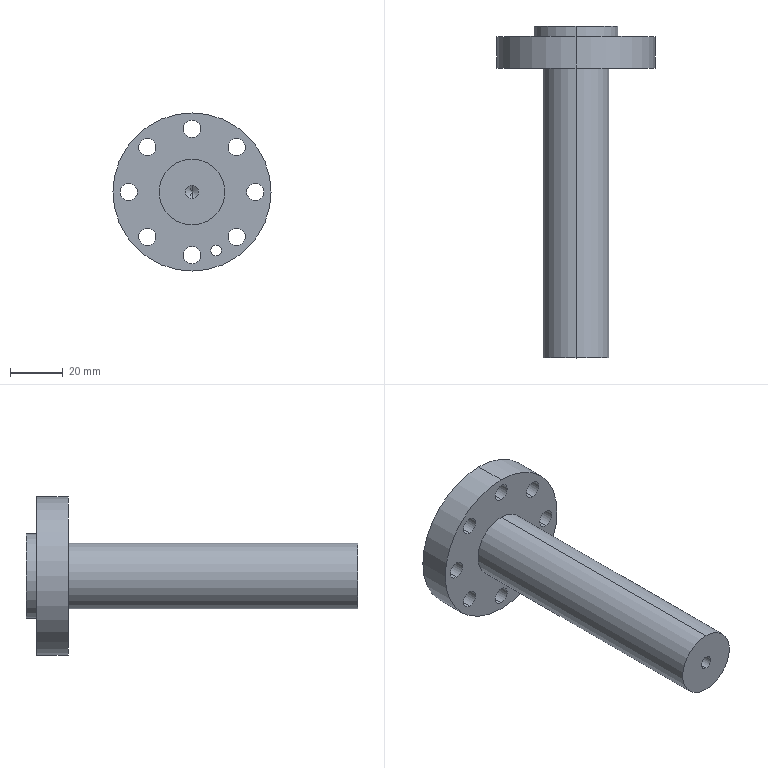Part | SolidWorks | features HoleWzd 3, Cut 1, Extrusion 1, ICE 1 | 1 solid | 32 faces | box 60 x 126 x 60 mm | volume 87403 mm3 | cylinder 26 | plane 4 | cone 2 | commonest cylinder face diameters 6.6 x16 4 x2 5 x2 25 x2 32 x2 60 x2
STEP:
#1=CARTESIAN_POINT('',(0.,15.,2.5));
#2=VERTEX_POINT('',#1);
#3=CARTESIAN_POINT('',(0.,15.,-2.5));
#4=VERTEX_POINT('',#3);
#5=CARTESIAN_POINT('',(0.,15.,0.));
#6=DIRECTION('',(0.,-1.,0.));
#7=DIRECTION('',(0.,0.,-1.));
#8=AXIS2_PLACEMENT_3D('',#5,#6,#7);
#9=CIRCLE('',#8,2.5);
#10=EDGE_CURVE('',#2,#4,#9,.T.);
#11=ORIENTED_EDGE('',*,*,#10,.F.);
#12=CARTESIAN_POINT('',(0.,0.,2.5));
#13=VERTEX_POINT('',#12);
#14=CARTESIAN_POINT('',(0.,0.,2.5));
#15=DIRECTION('',(0.,-1.,0.));
#16=VECTOR('',#15,1000.);
#17=LINE('',#14,#16);
#18=EDGE_CURVE('',#2,#13,#17,.T.);
#19=ORIENTED_EDGE('',*,*,#18,.T.);
#20=CARTESIAN_POINT('',(0.,0.,-2.5));
#21=VERTEX_POINT('',#20);
#22=CARTESIAN_POINT('',(0.,0.,0.));
#23=DIRECTION('',(0.,-1.,0.));
#24=DIRECTION('',(0.,0.,-1.));
#25=AXIS2_PLACEMENT_3D('',#22,#23,#24);
#26=CIRCLE('',#25,2.5);
#27=EDGE_CURVE('',#13,#21,#26,.T.);
#28=ORIENTED_EDGE('',*,*,#27,.T.);
#29=CARTESIAN_POINT('',(0.,0.,-2.5));
#30=DIRECTION('',(0.,-1.,0.));
#31=VECTOR('',#30,1000.);
#32=LINE('',#29,#31);
#33=EDGE_CURVE('',#4,#21,#32,.T.);
#34=ORIENTED_EDGE('',*,*,#33,.F.);
#35=EDGE_LOOP('',(#11,#19,#28,#34));
#36=FACE_OUTER_BOUND('',#35,.T.);
#37=CARTESIAN_POINT('',(0.,0.,0.));
#38=DIRECTION('',(0.,-1.,0.));
#39=DIRECTION('',(0.,0.,-1.));
#40=AXIS2_PLACEMENT_3D('',#37,#38,#39);
#41=CYLINDRICAL_SURFACE('',#40,2.5);
#42=ADVANCED_FACE('',(#36),#41,.F.);
#43=CARTESIAN_POINT('',(0.,16.502,0.));
#44=VERTEX_POINT('',#43);
#45=CARTESIAN_POINT('',(0.,15.,-2.5));
#46=DIRECTION('',(0.,-0.515,-0.8572));
#47=VECTOR('',#46,1000.);
#48=LINE('',#45,#47);
#49=EDGE_CURVE('',#44,#4,#48,.T.);
#50=ORIENTED_EDGE('',*,*,#49,.F.);
#51=CARTESIAN_POINT('',(0.,15.,2.5));
#52=DIRECTION('',(0.,-0.515,0.8572));
#53=VECTOR('',#52,1000.);
#54=LINE('',#51,#53);
#55=EDGE_CURVE('',#44,#2,#54,.T.);
#56=ORIENTED_EDGE('',*,*,#55,.T.);
#57=ORIENTED_EDGE('',*,*,#10,.T.);
#58=EDGE_LOOP('',(#50,#56,#57));
#59=FACE_OUTER_BOUND('',#58,.T.);
#60=CARTESIAN_POINT('',(0.,15.,0.));
#61=DIRECTION('',(0.,-1.,0.));
#62=DIRECTION('',(0.,0.,-1.));
#63=AXIS2_PLACEMENT_3D('',#60,#61,#62);
#64=CONICAL_SURFACE('',#63,2.5,1.03);
#65=ADVANCED_FACE('',(#59),#64,.F.);
#66=CARTESIAN_POINT('',(9.184,122.,-24.173));
#67=VERTEX_POINT('',#66);
#68=CARTESIAN_POINT('',(9.184,122.,-20.173));
#69=VERTEX_POINT('',#68);
#70=CARTESIAN_POINT('',(9.184,122.,-22.173));
#71=DIRECTION('',(0.,1.,0.));
#72=DIRECTION('',(0.,0.,1.));
#73=AXIS2_PLACEMENT_3D('',#70,#71,#72);
#74=CIRCLE('',#73,2.);
#75=EDGE_CURVE('',#67,#69,#74,.T.);
#76=ORIENTED_EDGE('',*,*,#75,.T.);
#77=CARTESIAN_POINT('',(9.184,110.,-20.173));
#78=VERTEX_POINT('',#77);
#79=CARTESIAN_POINT('',(9.184,110.,-20.173));
#80=DIRECTION('',(0.,-1.,0.));
#81=VECTOR('',#80,1000.);
#82=LINE('',#79,#81);
#83=EDGE_CURVE('',#69,#78,#82,.T.);
#84=ORIENTED_EDGE('',*,*,#83,.T.);
#85=CARTESIAN_POINT('',(9.184,110.,-24.173));
#86=VERTEX_POINT('',#85);
#87=CARTESIAN_POINT('',(9.184,110.,-22.173));
#88=DIRECTION('',(0.,-1.,0.));
#89=DIRECTION('',(0.,0.,-1.));
#90=AXIS2_PLACEMENT_3D('',#87,#88,#89);
#91=CIRCLE('',#90,2.);
#92=EDGE_CURVE('',#78,#86,#91,.T.);
#93=ORIENTED_EDGE('',*,*,#92,.T.);
#94=CARTESIAN_POINT('',(9.184,110.,-24.173));
#95=DIRECTION('',(0.,-1.,0.));
#96=VECTOR('',#95,1000.);
#97=LINE('',#94,#96);
#98=EDGE_CURVE('',#67,#86,#97,.T.);
#99=ORIENTED_EDGE('',*,*,#98,.F.);
#100=EDGE_LOOP('',(#76,#84,#93,#99));
#101=FACE_OUTER_BOUND('',#100,.T.);
#102=CARTESIAN_POINT('',(9.184,110.,-22.173));
#103=DIRECTION('',(0.,-1.,0.));
#104=DIRECTION('',(0.,0.,-1.));
#105=AXIS2_PLACEMENT_3D('',#102,#103,#104);
#106=CYLINDRICAL_SURFACE('',#105,2.);
#107=ADVANCED_FACE('',(#101),#106,.F.);
#108=CARTESIAN_POINT('',(0.,126.,16.));
#109=VERTEX_POINT('',#108);
#110=CARTESIAN_POINT('',(0.,126.,-16.));
#111=VERTEX_POINT('',#110);
#112=CARTESIAN_POINT('',(0.,126.,0.));
#113=DIRECTION('',(0.,1.,0.));
#114=DIRECTION('',(0.,0.,1.));
#115=AXIS2_PLACEMENT_3D('',#112,#113,#114);
#116=CIRCLE('',#115,16.);
#117=EDGE_CURVE('',#109,#111,#116,.T.);
#118=ORIENTED_EDGE('',*,*,#117,.F.);
#119=CARTESIAN_POINT('',(0.,122.,16.));
#120=VERTEX_POINT('',#119);
#121=CARTESIAN_POINT('',(0.,126.,16.));
#122=DIRECTION('',(0.,-1.,0.));
#123=VECTOR('',#122,1000.);
#124=LINE('',#121,#123);
#125=EDGE_CURVE('',#109,#120,#124,.T.);
#126=ORIENTED_EDGE('',*,*,#125,.T.);
#127=CARTESIAN_POINT('',(0.,122.,-16.));
#128=VERTEX_POINT('',#127);
#129=CARTESIAN_POINT('',(0.,122.,0.));
#130=DIRECTION('',(0.,1.,0.));
#131=DIRECTION('',(0.,0.,1.));
#132=AXIS2_PLACEMENT_3D('',#129,#130,#131);
#133=CIRCLE('',#132,16.);
#134=EDGE_CURVE('',#120,#128,#133,.T.);
#135=ORIENTED_EDGE('',*,*,#134,.T.);
#136=CARTESIAN_POINT('',(0.,126.,-16.));
#137=DIRECTION('',(0.,-1.,0.));
#138=VECTOR('',#137,1000.);
#139=LINE('',#136,#138);
#140=EDGE_CURVE('',#111,#128,#139,.T.);
#141=ORIENTED_EDGE('',*,*,#140,.F.);
#142=EDGE_LOOP('',(#118,#126,#135,#141));
#143=FACE_OUTER_BOUND('',#142,.T.);
#144=CARTESIAN_POINT('',(0.,126.,0.));
#145=DIRECTION('',(0.,-1.,0.));
#146=DIRECTION('',(0.,0.,-1.));
#147=AXIS2_PLACEMENT_3D('',#144,#145,#146);
#148=CYLINDRICAL_SURFACE('',#147,16.);
#149=ADVANCED_FACE('',(#143),#148,.T.);
#150=CARTESIAN_POINT('',(24.,122.,3.3));
#151=VERTEX_POINT('',#150);
#152=CARTESIAN_POINT('',(24.,122.,-3.3));
#153=VERTEX_POINT('',#152);
#154=CARTESIAN_POINT('',(24.,122.,0.));
#155=DIRECTION('',(0.,-1.,0.));
#156=DIRECTION('',(0.,0.,-1.));
#157=AXIS2_PLACEMENT_3D('',#154,#155,#156);
#158=CIRCLE('',#157,3.3);
#159=EDGE_CURVE('',#151,#153,#158,.T.);
#160=ORIENTED_EDGE('',*,*,#159,.F.);
#161=CARTESIAN_POINT('',(24.,110.,3.3));
#162=VERTEX_POINT('',#161);
#163=CARTESIAN_POINT('',(24.,110.,3.3));
#164=DIRECTION('',(0.,-1.,0.));
#165=VECTOR('',#164,1000.);
#166=LINE('',#163,#165);
#167=EDGE_CURVE('',#151,#162,#166,.T.);
#168=ORIENTED_EDGE('',*,*,#167,.T.);
#169=CARTESIAN_POINT('',(24.,110.,-3.3));
#170=VERTEX_POINT('',#169);
#171=CARTESIAN_POINT('',(24.,110.,0.));
#172=DIRECTION('',(0.,-1.,0.));
#173=DIRECTION('',(0.,0.,-1.));
#174=AXIS2_PLACEMENT_3D('',#171,#172,#173);
#175=CIRCLE('',#174,3.3);
#176=EDGE_CURVE('',#162,#170,#175,.T.);
#177=ORIENTED_EDGE('',*,*,#176,.T.);
#178=CARTESIAN_POINT('',(24.,110.,-3.3));
#179=DIRECTION('',(0.,-1.,0.));
#180=VECTOR('',#179,1000.);
#181=LINE('',#178,#180);
#182=EDGE_CURVE('',#153,#170,#181,.T.);
#183=ORIENTED_EDGE('',*,*,#182,.F.);
#184=EDGE_LOOP('',(#160,#168,#177,#183));
#185=FACE_OUTER_BOUND('',#184,.T.);
#186=CARTESIAN_POINT('',(24.,110.,0.));
#187=DIRECTION('',(0.,-1.,0.));
#188=DIRECTION('',(0.,0.,-1.));
#189=AXIS2_PLACEMENT_3D('',#186,#187,#188);
#190=CYLINDRICAL_SURFACE('',#189,3.3);
#191=ADVANCED_FACE('',(#185),#190,.F.);
#192=CARTESIAN_POINT('',(16.971,122.,-13.671));
#193=VERTEX_POINT('',#192);
#194=CARTESIAN_POINT('',(16.971,122.,-20.271));
#195=VERTEX_POINT('',#194);
#196=CARTESIAN_POINT('',(16.971,122.,-16.971));
#197=DIRECTION('',(0.,-1.,0.));
#198=DIRECTION('',(0.,0.,-1.));
#199=AXIS2_PLACEMENT_3D('',#196,#197,#198);
#200=CIRCLE('',#199,3.3);
#201=EDGE_CURVE('',#193,#195,#200,.T.);
#202=ORIENTED_EDGE('',*,*,#201,.F.);
#203=CARTESIAN_POINT('',(16.971,110.,-13.671));
#204=VERTEX_POINT('',#203);
#205=CARTESIAN_POINT('',(16.971,110.,-13.671));
#206=DIRECTION('',(0.,-1.,0.));
#207=VECTOR('',#206,1000.);
#208=LINE('',#205,#207);
#209=EDGE_CURVE('',#193,#204,#208,.T.);
#210=ORIENTED_EDGE('',*,*,#209,.T.);
#211=CARTESIAN_POINT('',(16.971,110.,-20.271));
#212=VERTEX_POINT('',#211);
#213=CARTESIAN_POINT('',(16.971,110.,-16.971));
#214=DIRECTION('',(0.,-1.,0.));
#215=DIRECTION('',(0.,0.,-1.));
#216=AXIS2_PLACEMENT_3D('',#213,#214,#215);
#217=CIRCLE('',#216,3.3);
#218=EDGE_CURVE('',#204,#212,#217,.T.);
#219=ORIENTED_EDGE('',*,*,#218,.T.);
#220=CARTESIAN_POINT('',(16.971,110.,-20.271));
#221=DIRECTION('',(0.,-1.,0.));
#222=VECTOR('',#221,1000.);
#223=LINE('',#220,#222);
#224=EDGE_CURVE('',#195,#212,#223,.T.);
#225=ORIENTED_EDGE('',*,*,#224,.F.);
#226=EDGE_LOOP('',(#202,#210,#219,#225));
#227=FACE_OUTER_BOUND('',#226,.T.);
#228=CARTESIAN_POINT('',(16.971,110.,-16.971));
#229=DIRECTION('',(0.,-1.,0.));
#230=DIRECTION('',(0.,0.,-1.));
#231=AXIS2_PLACEMENT_3D('',#228,#229,#230);
#232=CYLINDRICAL_SURFACE('',#231,3.3);
#233=ADVANCED_FACE('',(#227),#232,.F.);
#234=CARTESIAN_POINT('',(0.,122.,-20.7));
#235=VERTEX_POINT('',#234);
#236=CARTESIAN_POINT('',(0.,122.,-27.3));
#237=VERTEX_POINT('',#236);
#238=CARTESIAN_POINT('',(0.,122.,-24.));
#239=DIRECTION('',(0.,-1.,0.));
#240=DIRECTION('',(0.,0.,-1.));
#241=AXIS2_PLACEMENT_3D('',#238,#239,#240);
#242=CIRCLE('',#241,3.3);
#243=EDGE_CURVE('',#235,#237,#242,.T.);
#244=ORIENTED_EDGE('',*,*,#243,.F.);
#245=CARTESIAN_POINT('',(0.,110.,-20.7));
#246=VERTEX_POINT('',#245);
#247=CARTESIAN_POINT('',(0.,110.,-20.7));
#248=DIRECTION('',(0.,-1.,0.));
#249=VECTOR('',#248,1000.);
#250=LINE('',#247,#249);
#251=EDGE_CURVE('',#235,#246,#250,.T.);
#252=ORIENTED_EDGE('',*,*,#251,.T.);
#253=CARTESIAN_POINT('',(0.,110.,-27.3));
#254=VERTEX_POINT('',#253);
#255=CARTESIAN_POINT('',(0.,110.,-24.));
#256=DIRECTION('',(0.,-1.,0.));
#257=DIRECTION('',(0.,0.,-1.));
#258=AXIS2_PLACEMENT_3D('',#255,#256,#257);
#259=CIRCLE('',#258,3.3);
#260=EDGE_CURVE('',#246,#254,#259,.T.);
#261=ORIENTED_EDGE('',*,*,#260,.T.);
#262=CARTESIAN_POINT('',(0.,110.,-27.3));
#263=DIRECTION('',(0.,-1.,0.));
#264=VECTOR('',#263,1000.);
#265=LINE('',#262,#264);
#266=EDGE_CURVE('',#237,#254,#265,.T.);
#267=ORIENTED_EDGE('',*,*,#266,.F.);
#268=EDGE_LOOP('',(#244,#252,#261,#267));
#269=FACE_OUTER_BOUND('',#268,.T.);
#270=CARTESIAN_POINT('',(0.,110.,-24.));
#271=DIRECTION('',(0.,-1.,0.));
#272=DIRECTION('',(0.,0.,-1.));
#273=AXIS2_PLACEMENT_3D('',#270,#271,#272);
#274=CYLINDRICAL_SURFACE('',#273,3.3);
#275=ADVANCED_FACE('',(#269),#274,.F.);
#276=CARTESIAN_POINT('',(-16.971,122.,-13.671));
#277=VERTEX_POINT('',#276);
#278=CARTESIAN_POINT('',(-16.971,122.,-20.271));
#279=VERTEX_POINT('',#278);
#280=CARTESIAN_POINT('',(-16.971,122.,-16.971));
#281=DIRECTION('',(0.,-1.,0.));
#282=DIRECTION('',(0.,0.,-1.));
#283=AXIS2_PLACEMENT_3D('',#280,#281,#282);
#284=CIRCLE('',#283,3.3);
#285=EDGE_CURVE('',#277,#279,#284,.T.);
#286=ORIENTED_EDGE('',*,*,#285,.F.);
#287=CARTESIAN_POINT('',(-16.971,110.,-13.671));
#288=VERTEX_POINT('',#287);
#289=CARTESIAN_POINT('',(-16.971,110.,-13.671));
#290=DIRECTION('',(0.,-1.,0.));
#291=VECTOR('',#290,1000.);
#292=LINE('',#289,#291);
#293=EDGE_CURVE('',#277,#288,#292,.T.);
#294=ORIENTED_EDGE('',*,*,#293,.T.);
#295=CARTESIAN_POINT('',(-16.971,110.,-20.271));
#296=VERTEX_POINT('',#295);
#297=CARTESIAN_POINT('',(-16.971,110.,-16.971));
#298=DIRECTION('',(0.,-1.,0.));
#299=DIRECTION('',(0.,0.,-1.));
#300=AXIS2_PLACEMENT_3D('',#297,#298,#299);
#301=CIRCLE('',#300,3.3);
#302=EDGE_CURVE('',#288,#296,#301,.T.);
#303=ORIENTED_EDGE('',*,*,#302,.T.);
#304=CARTESIAN_POINT('',(-16.971,110.,-20.271));
#305=DIRECTION('',(0.,-1.,0.));
#306=VECTOR('',#305,1000.);
#307=LINE('',#304,#306);
#308=EDGE_CURVE('',#279,#296,#307,.T.);
#309=ORIENTED_EDGE('',*,*,#308,.F.);
#310=EDGE_LOOP('',(#286,#294,#303,#309));
#311=FACE_OUTER_BOUND('',#310,.T.);
#312=CARTESIAN_POINT('',(-16.971,110.,-16.971));
#313=DIRECTION('',(0.,-1.,0.));
#314=DIRECTION('',(0.,0.,-1.));
#315=AXIS2_PLACEMENT_3D('',#312,#313,#314);
#316=CYLINDRICAL_SURFACE('',#315,3.3);
#317=ADVANCED_FACE('',(#311),#316,.F.);
#318=CARTESIAN_POINT('',(-24.,122.,3.3));
#319=VERTEX_POINT('',#318);
#320=CARTESIAN_POINT('',(-24.,122.,-3.3));
#321=VERTEX_POINT('',#320);
#322=CARTESIAN_POINT('',(-24.,122.,0.));
#323=DIRECTION('',(0.,-1.,0.));
#324=DIRECTION('',(0.,0.,-1.));
#325=AXIS2_PLACEMENT_3D('',#322,#323,#324);
#326=CIRCLE('',#325,3.3);
#327=EDGE_CURVE('',#319,#321,#326,.T.);
#328=ORIENTED_EDGE('',*,*,#327,.F.);
#329=CARTESIAN_POINT('',(-24.,110.,3.3));
#330=VERTEX_POINT('',#329);
#331=CARTESIAN_POINT('',(-24.,110.,3.3));
#332=DIRECTION('',(0.,-1.,0.));
#333=VECTOR('',#332,1000.);
#334=LINE('',#331,#333);
#335=EDGE_CURVE('',#319,#330,#334,.T.);
#336=ORIENTED_EDGE('',*,*,#335,.T.);
#337=CARTESIAN_POINT('',(-24.,110.,-3.3));
#338=VERTEX_POINT('',#337);
#339=CARTESIAN_POINT('',(-24.,110.,0.));
#340=DIRECTION('',(0.,-1.,0.));
#341=DIRECTION('',(0.,0.,-1.));
#342=AXIS2_PLACEMENT_3D('',#339,#340,#341);
#343=CIRCLE('',#342,3.3);
#344=EDGE_CURVE('',#330,#338,#343,.T.);
#345=ORIENTED_EDGE('',*,*,#344,.T.);
#346=CARTESIAN_POINT('',(-24.,110.,-3.3));
#347=DIRECTION('',(0.,-1.,0.));
#348=VECTOR('',#347,1000.);
#349=LINE('',#346,#348);
#350=EDGE_CURVE('',#321,#338,#349,.T.);
#351=ORIENTED_EDGE('',*,*,#350,.F.);
#352=EDGE_LOOP('',(#328,#336,#345,#351));
#353=FACE_OUTER_BOUND('',#352,.T.);
#354=CARTESIAN_POINT('',(-24.,110.,0.));
#355=DIRECTION('',(0.,-1.,0.));
#356=DIRECTION('',(0.,0.,-1.));
#357=AXIS2_PLACEMENT_3D('',#354,#355,#356);
#358=CYLINDRICAL_SURFACE('',#357,3.3);
#359=ADVANCED_FACE('',(#353),#358,.F.);
#360=CARTESIAN_POINT('',(-16.971,122.,20.271));
#361=VERTEX_POINT('',#360);
#362=CARTESIAN_POINT('',(-16.971,122.,13.671));
#363=VERTEX_POINT('',#362);
#364=CARTESIAN_POINT('',(-16.971,122.,16.971));
#365=DIRECTION('',(0.,-1.,0.));
#366=DIRECTION('',(0.,0.,-1.));
#367=AXIS2_PLACEMENT_3D('',#364,#365,#366);
#368=CIRCLE('',#367,3.3);
#369=EDGE_CURVE('',#361,#363,#368,.T.);
#370=ORIENTED_EDGE('',*,*,#369,.F.);
#371=CARTESIAN_POINT('',(-16.971,110.,20.271));
#372=VERTEX_POINT('',#371);
#373=CARTESIAN_POINT('',(-16.971,110.,20.271));
#374=DIRECTION('',(0.,-1.,0.));
#375=VECTOR('',#374,1000.);
#376=LINE('',#373,#375);
#377=EDGE_CURVE('',#361,#372,#376,.T.);
#378=ORIENTED_EDGE('',*,*,#377,.T.);
#379=CARTESIAN_POINT('',(-16.971,110.,13.671));
#380=VERTEX_POINT('',#379);
#381=CARTESIAN_POINT('',(-16.971,110.,16.971));
#382=DIRECTION('',(0.,-1.,0.));
#383=DIRECTION('',(0.,0.,-1.));
#384=AXIS2_PLACEMENT_3D('',#381,#382,#383);
#385=CIRCLE('',#384,3.3);
#386=EDGE_CURVE('',#372,#380,#385,.T.);
#387=ORIENTED_EDGE('',*,*,#386,.T.);
#388=CARTESIAN_POINT('',(-16.971,110.,13.671));
#389=DIRECTION('',(0.,-1.,0.));
#390=VECTOR('',#389,1000.);
#391=LINE('',#388,#390);
#392=EDGE_CURVE('',#363,#380,#391,.T.);
#393=ORIENTED_EDGE('',*,*,#392,.F.);
#394=EDGE_LOOP('',(#370,#378,#387,#393));
#395=FACE_OUTER_BOUND('',#394,.T.);
#396=CARTESIAN_POINT('',(-16.971,110.,16.971));
#397=DIRECTION('',(0.,-1.,0.));
#398=DIRECTION('',(0.,0.,-1.));
#399=AXIS2_PLACEMENT_3D('',#396,#397,#398);
#400=CYLINDRICAL_SURFACE('',#399,3.3);
#401=ADVANCED_FACE('',(#395),#400,.F.);
#402=CARTESIAN_POINT('',(0.,122.,27.3));
#403=VERTEX_POINT('',#402);
#404=CARTESIAN_POINT('',(0.,122.,20.7));
#405=VERTEX_POINT('',#404);
#406=CARTESIAN_POINT('',(0.,122.,24.));
#407=DIRECTION('',(0.,-1.,0.));
#408=DIRECTION('',(0.,0.,-1.));
#409=AXIS2_PLACEMENT_3D('',#406,#407,#408);
#410=CIRCLE('',#409,3.3);
#411=EDGE_CURVE('',#403,#405,#410,.T.);
#412=ORIENTED_EDGE('',*,*,#411,.F.);
#413=CARTESIAN_POINT('',(0.,110.,27.3));
#414=VERTEX_POINT('',#413);
#415=CARTESIAN_POINT('',(0.,110.,27.3));
#416=DIRECTION('',(0.,-1.,0.));
#417=VECTOR('',#416,1000.);
#418=LINE('',#415,#417);
#419=EDGE_CURVE('',#403,#414,#418,.T.);
#420=ORIENTED_EDGE('',*,*,#419,.T.);
#421=CARTESIAN_POINT('',(0.,110.,20.7));
#422=VERTEX_POINT('',#421);
#423=CARTESIAN_POINT('',(0.,110.,24.));
#424=DIRECTION('',(0.,-1.,0.));
#425=DIRECTION('',(0.,0.,-1.));
#426=AXIS2_PLACEMENT_3D('',#423,#424,#425);
#427=CIRCLE('',#426,3.3);
#428=EDGE_CURVE('',#414,#422,#427,.T.);
#429=ORIENTED_EDGE('',*,*,#428,.T.);
#430=CARTESIAN_POINT('',(0.,110.,20.7));
#431=DIRECTION('',(0.,-1.,0.));
#432=VECTOR('',#431,1000.);
#433=LINE('',#430,#432);
#434=EDGE_CURVE('',#405,#422,#433,.T.);
#435=ORIENTED_EDGE('',*,*,#434,.F.);
#436=EDGE_LOOP('',(#412,#420,#429,#435));
#437=FACE_OUTER_BOUND('',#436,.T.);
#438=CARTESIAN_POINT('',(0.,110.,24.));
#439=DIRECTION('',(0.,-1.,0.));
#440=DIRECTION('',(0.,0.,-1.));
#441=AXIS2_PLACEMENT_3D('',#438,#439,#440);
#442=CYLINDRICAL_SURFACE('',#441,3.3);
#443=ADVANCED_FACE('',(#437),#442,.F.);
#444=CARTESIAN_POINT('',(16.971,122.,20.271));
#445=VERTEX_POINT('',#444);
#446=CARTESIAN_POINT('',(16.971,122.,13.671));
#447=VERTEX_POINT('',#446);
#448=CARTESIAN_POINT('',(16.971,122.,16.971));
#449=DIRECTION('',(0.,-1.,0.));
#450=DIRECTION('',(0.,0.,-1.));
#451=AXIS2_PLACEMENT_3D('',#448,#449,#450);
#452=CIRCLE('',#451,3.3);
#453=EDGE_CURVE('',#445,#447,#452,.T.);
#454=ORIENTED_EDGE('',*,*,#453,.F.);
#455=CARTESIAN_POINT('',(16.971,110.,20.271));
#456=VERTEX_POINT('',#455);
#457=CARTESIAN_POINT('',(16.971,110.,20.271));
#458=DIRECTION('',(0.,-1.,0.));
#459=VECTOR('',#458,1000.);
#460=LINE('',#457,#459);
#461=EDGE_CURVE('',#445,#456,#460,.T.);
#462=ORIENTED_EDGE('',*,*,#461,.T.);
#463=CARTESIAN_POINT('',(16.971,110.,13.671));
#464=VERTEX_POINT('',#463);
#465=CARTESIAN_POINT('',(16.971,110.,16.971));
#466=DIRECTION('',(0.,-1.,0.));
#467=DIRECTION('',(0.,0.,-1.));
#468=AXIS2_PLACEMENT_3D('',#465,#466,#467);
#469=CIRCLE('',#468,3.3);
#470=EDGE_CURVE('',#456,#464,#469,.T.);
#471=ORIENTED_EDGE('',*,*,#470,.T.);
#472=CARTESIAN_POINT('',(16.971,110.,13.671));
#473=DIRECTION('',(0.,-1.,0.));
#474=VECTOR('',#473,1000.);
#475=LINE('',#472,#474);
#476=EDGE_CURVE('',#447,#464,#475,.T.);
#477=ORIENTED_EDGE('',*,*,#476,.F.);
#478=EDGE_LOOP('',(#454,#462,#471,#477));
#479=FACE_OUTER_BOUND('',#478,.T.);
#480=CARTESIAN_POINT('',(16.971,110.,16.971));
#481=DIRECTION('',(0.,-1.,0.));
#482=DIRECTION('',(0.,0.,-1.));
#483=AXIS2_PLACEMENT_3D('',#480,#481,#482);
#484=CYLINDRICAL_SURFACE('',#483,3.3);
#485=ADVANCED_FACE('',(#479),#484,.F.);
#486=CARTESIAN_POINT('',(0.,0.,12.5));
#487=VERTEX_POINT('',#486);
#488=CARTESIAN_POINT('',(0.,0.,-12.5));
#489=VERTEX_POINT('',#488);
#490=CARTESIAN_POINT('',(0.,0.,0.));
#491=DIRECTION('',(0.,1.,0.));
#492=DIRECTION('',(0.,0.,1.));
#493=AXIS2_PLACEMENT_3D('',#490,#491,#492);
#494=CIRCLE('',#493,12.5);
#495=EDGE_CURVE('',#487,#489,#494,.T.);
#496=ORIENTED_EDGE('',*,*,#495,.T.);
#497=CARTESIAN_POINT('',(0.,110.,-12.5));
#498=VERTEX_POINT('',#497);
#499=CARTESIAN_POINT('',(0.,0.,-12.5));
#500=DIRECTION('',(0.,1.,0.));
#501=VECTOR('',#500,1000.);
#502=LINE('',#499,#501);
#503=EDGE_CURVE('',#489,#498,#502,.T.);
#504=ORIENTED_EDGE('',*,*,#503,.T.);
#505=CARTESIAN_POINT('',(0.,110.,12.5));
#506=VERTEX_POINT('',#505);
#507=CARTESIAN_POINT('',(0.,110.,0.));
#508=DIRECTION('',(0.,1.,0.));
#509=DIRECTION('',(0.,0.,1.));
#510=AXIS2_PLACEMENT_3D('',#507,#508,#509);
#511=CIRCLE('',#510,12.5);
#512=EDGE_CURVE('',#506,#498,#511,.T.);
#513=ORIENTED_EDGE('',*,*,#512,.F.);
#514=CARTESIAN_POINT('',(0.,0.,12.5));
#515=DIRECTION('',(0.,1.,0.));
#516=VECTOR('',#515,1000.);
#517=LINE('',#514,#516);
#518=EDGE_CURVE('',#487,#506,#517,.T.);
#519=ORIENTED_EDGE('',*,*,#518,.F.);
#520=EDGE_LOOP('',(#496,#504,#513,#519));
#521=FACE_OUTER_BOUND('',#520,.T.);
#522=CARTESIAN_POINT('',(0.,0.,0.));
#523=DIRECTION('',(0.,1.,0.));
#524=DIRECTION('',(0.,0.,1.));
#525=AXIS2_PLACEMENT_3D('',#522,#523,#524);
#526=CYLINDRICAL_SURFACE('',#525,12.5);
#527=ADVANCED_FACE('',(#521),#526,.T.);
#528=CARTESIAN_POINT('',(0.,122.,30.));
#529=VERTEX_POINT('',#528);
#530=CARTESIAN_POINT('',(0.,122.,-30.));
#531=VERTEX_POINT('',#530);
#532=CARTESIAN_POINT('',(0.,122.,0.));
#533=DIRECTION('',(0.,1.,0.));
#534=DIRECTION('',(0.,0.,1.));
#535=AXIS2_PLACEMENT_3D('',#532,#533,#534);
#536=CIRCLE('',#535,30.);
#537=EDGE_CURVE('',#529,#531,#536,.T.);
#538=ORIENTED_EDGE('',*,*,#537,.F.);
#539=CARTESIAN_POINT('',(0.,110.,30.));
#540=VERTEX_POINT('',#539);
#541=CARTESIAN_POINT('',(0.,122.,30.));
#542=DIRECTION('',(0.,-1.,0.));
#543=VECTOR('',#542,1000.);
#544=LINE('',#541,#543);
#545=EDGE_CURVE('',#529,#540,#544,.T.);
#546=ORIENTED_EDGE('',*,*,#545,.T.);
#547=CARTESIAN_POINT('',(0.,110.,-30.));
#548=VERTEX_POINT('',#547);
#549=CARTESIAN_POINT('',(0.,110.,0.));
#550=DIRECTION('',(0.,1.,0.));
#551=DIRECTION('',(0.,0.,1.));
#552=AXIS2_PLACEMENT_3D('',#549,#550,#551);
#553=CIRCLE('',#552,30.);
#554=EDGE_CURVE('',#540,#548,#553,.T.);
#555=ORIENTED_EDGE('',*,*,#554,.T.);
#556=CARTESIAN_POINT('',(0.,122.,-30.));
#557=DIRECTION('',(0.,-1.,0.));
#558=VECTOR('',#557,1000.);
#559=LINE('',#556,#558);
#560=EDGE_CURVE('',#531,#548,#559,.T.);
#561=ORIENTED_EDGE('',*,*,#560,.F.);
#562=EDGE_LOOP('',(#538,#546,#555,#561));
#563=FACE_OUTER_BOUND('',#562,.T.);
#564=CARTESIAN_POINT('',(0.,122.,0.));
#565=DIRECTION('',(0.,-1.,0.));
#566=DIRECTION('',(0.,0.,-1.));
#567=AXIS2_PLACEMENT_3D('',#564,#565,#566);
#568=CYLINDRICAL_SURFACE('',#567,30.);
#569=ADVANCED_FACE('',(#563),#568,.T.);
#570=ORIENTED_EDGE('',*,*,#545,.F.);
#571=CARTESIAN_POINT('',(0.,122.,0.));
#572=DIRECTION('',(0.,1.,0.));
#573=DIRECTION('',(0.,0.,1.));
#574=AXIS2_PLACEMENT_3D('',#571,#572,#573);
#575=CIRCLE('',#574,30.);
#576=EDGE_CURVE('',#531,#529,#575,.T.);
#577=ORIENTED_EDGE('',*,*,#576,.F.);
#578=ORIENTED_EDGE('',*,*,#560,.T.);
#579=CARTESIAN_POINT('',(0.,110.,0.));
#580=DIRECTION('',(0.,1.,0.));
#581=DIRECTION('',(0.,0.,1.));
#582=AXIS2_PLACEMENT_3D('',#579,#580,#581);
#583=CIRCLE('',#582,30.);
#584=EDGE_CURVE('',#548,#540,#583,.T.);
#585=ORIENTED_EDGE('',*,*,#584,.T.);
#586=EDGE_LOOP('',(#570,#577,#578,#585));
#587=FACE_OUTER_BOUND('',#586,.T.);
#588=CARTESIAN_POINT('',(0.,122.,0.));
#589=DIRECTION('',(0.,-1.,0.));
#590=DIRECTION('',(0.,0.,-1.));
#591=AXIS2_PLACEMENT_3D('',#588,#589,#590);
#592=CYLINDRICAL_SURFACE('',#591,30.);
#593=ADVANCED_FACE('',(#587),#592,.T.);
#594=ORIENTED_EDGE('',*,*,#75,.F.);
#595=CARTESIAN_POINT('',(9.184,122.,-22.173));
#596=DIRECTION('',(0.,1.,0.));
#597=DIRECTION('',(0.,0.,1.));
#598=AXIS2_PLACEMENT_3D('',#595,#596,#597);
#599=CIRCLE('',#598,2.);
#600=EDGE_CURVE('',#69,#67,#599,.T.);
#601=ORIENTED_EDGE('',*,*,#600,.F.);
#602=EDGE_LOOP('',(#594,#601));
#603=FACE_BOUND('',#602,.T.);
#604=CARTESIAN_POINT('',(0.,122.,0.));
#605=DIRECTION('',(0.,1.,0.));
#606=DIRECTION('',(0.,0.,1.));
#607=AXIS2_PLACEMENT_3D('',#604,#605,#606);
#608=CIRCLE('',#607,16.);
#609=EDGE_CURVE('',#128,#120,#608,.T.);
#610=ORIENTED_EDGE('',*,*,#609,.F.);
#611=ORIENTED_EDGE('',*,*,#134,.F.);
#612=EDGE_LOOP('',(#610,#611));
#613=FACE_BOUND('',#612,.T.);
#614=CARTESIAN_POINT('',(24.,122.,0.));
#615=DIRECTION('',(0.,-1.,0.));
#616=DIRECTION('',(0.,0.,-1.));
#617=AXIS2_PLACEMENT_3D('',#614,#615,#616);
#618=CIRCLE('',#617,3.3);
#619=EDGE_CURVE('',#153,#151,#618,.T.);
#620=ORIENTED_EDGE('',*,*,#619,.T.);
#621=ORIENTED_EDGE('',*,*,#159,.T.);
#622=EDGE_LOOP('',(#620,#621));
#623=FACE_BOUND('',#622,.T.);
#624=CARTESIAN_POINT('',(16.971,122.,-16.971));
#625=DIRECTION('',(0.,-1.,0.));
#626=DIRECTION('',(0.,0.,-1.));
#627=AXIS2_PLACEMENT_3D('',#624,#625,#626);
#628=CIRCLE('',#627,3.3);
#629=EDGE_CURVE('',#195,#193,#628,.T.);
#630=ORIENTED_EDGE('',*,*,#629,.T.);
#631=ORIENTED_EDGE('',*,*,#201,.T.);
#632=EDGE_LOOP('',(#630,#631));
#633=FACE_BOUND('',#632,.T.);
#634=CARTESIAN_POINT('',(0.,122.,-24.));
#635=DIRECTION('',(0.,-1.,0.));
#636=DIRECTION('',(0.,0.,-1.));
#637=AXIS2_PLACEMENT_3D('',#634,#635,#636);
#638=CIRCLE('',#637,3.3);
#639=EDGE_CURVE('',#237,#235,#638,.T.);
#640=ORIENTED_EDGE('',*,*,#639,.T.);
#641=ORIENTED_EDGE('',*,*,#243,.T.);
#642=EDGE_LOOP('',(#640,#641));
#643=FACE_BOUND('',#642,.T.);
#644=CARTESIAN_POINT('',(-16.971,122.,-16.971));
#645=DIRECTION('',(0.,-1.,0.));
#646=DIRECTION('',(0.,0.,-1.));
#647=AXIS2_PLACEMENT_3D('',#644,#645,#646);
#648=CIRCLE('',#647,3.3);
#649=EDGE_CURVE('',#279,#277,#648,.T.);
#650=ORIENTED_EDGE('',*,*,#649,.T.);
#651=ORIENTED_EDGE('',*,*,#285,.T.);
#652=EDGE_LOOP('',(#650,#651));
#653=FACE_BOUND('',#652,.T.);
#654=CARTESIAN_POINT('',(-24.,122.,0.));
#655=DIRECTION('',(0.,-1.,0.));
#656=DIRECTION('',(0.,0.,-1.));
#657=AXIS2_PLACEMENT_3D('',#654,#655,#656);
#658=CIRCLE('',#657,3.3);
#659=EDGE_CURVE('',#321,#319,#658,.T.);
#660=ORIENTED_EDGE('',*,*,#659,.T.);
#661=ORIENTED_EDGE('',*,*,#327,.T.);
#662=EDGE_LOOP('',(#660,#661));
#663=FACE_BOUND('',#662,.T.);
#664=CARTESIAN_POINT('',(-16.971,122.,16.971));
#665=DIRECTION('',(0.,-1.,0.));
#666=DIRECTION('',(0.,0.,-1.));
#667=AXIS2_PLACEMENT_3D('',#664,#665,#666);
#668=CIRCLE('',#667,3.3);
#669=EDGE_CURVE('',#363,#361,#668,.T.);
#670=ORIENTED_EDGE('',*,*,#669,.T.);
#671=ORIENTED_EDGE('',*,*,#369,.T.);
#672=EDGE_LOOP('',(#670,#671));
#673=FACE_BOUND('',#672,.T.);
#674=CARTESIAN_POINT('',(0.,122.,24.));
#675=DIRECTION('',(0.,-1.,0.));
#676=DIRECTION('',(0.,0.,-1.));
#677=AXIS2_PLACEMENT_3D('',#674,#675,#676);
#678=CIRCLE('',#677,3.3);
#679=EDGE_CURVE('',#405,#403,#678,.T.);
#680=ORIENTED_EDGE('',*,*,#679,.T.);
#681=ORIENTED_EDGE('',*,*,#411,.T.);
#682=EDGE_LOOP('',(#680,#681));
#683=FACE_BOUND('',#682,.T.);
#684=CARTESIAN_POINT('',(16.971,122.,16.971));
#685=DIRECTION('',(0.,-1.,0.));
#686=DIRECTION('',(0.,0.,-1.));
#687=AXIS2_PLACEMENT_3D('',#684,#685,#686);
#688=CIRCLE('',#687,3.3);
#689=EDGE_CURVE('',#447,#445,#688,.T.);
#690=ORIENTED_EDGE('',*,*,#689,.T.);
#691=ORIENTED_EDGE('',*,*,#453,.T.);
#692=EDGE_LOOP('',(#690,#691));
#693=FACE_BOUND('',#692,.T.);
#694=ORIENTED_EDGE('',*,*,#576,.T.);
#695=ORIENTED_EDGE('',*,*,#537,.T.);
#696=EDGE_LOOP('',(#694,#695));
#697=FACE_OUTER_BOUND('',#696,.T.);
#698=CARTESIAN_POINT('',(0.,122.,0.));
#699=DIRECTION('',(0.,1.,0.));
#700=DIRECTION('',(0.,0.,1.));
#701=AXIS2_PLACEMENT_3D('',#698,#699,#700);
#702=PLANE('',#701);
#703=ADVANCED_FACE('',(#603,#613,#623,#633,#643,#653,#663,#673,#683,#693,#697),#702,.T.);
#704=CARTESIAN_POINT('',(9.184,110.,-22.173));
#705=DIRECTION('',(0.,-1.,0.));
#706=DIRECTION('',(0.,0.,-1.));
#707=AXIS2_PLACEMENT_3D('',#704,#705,#706);
#708=CIRCLE('',#707,2.);
#709=EDGE_CURVE('',#86,#78,#708,.T.);
#710=ORIENTED_EDGE('',*,*,#709,.F.);
#711=ORIENTED_EDGE('',*,*,#92,.F.);
#712=EDGE_LOOP('',(#710,#711));
#713=FACE_BOUND('',#712,.T.);
#714=CARTESIAN_POINT('',(24.,110.,0.));
#715=DIRECTION('',(0.,-1.,0.));
#716=DIRECTION('',(0.,0.,-1.));
#717=AXIS2_PLACEMENT_3D('',#714,#715,#716);
#718=CIRCLE('',#717,3.3);
#719=EDGE_CURVE('',#170,#162,#718,.T.);
#720=ORIENTED_EDGE('',*,*,#719,.F.);
#721=ORIENTED_EDGE('',*,*,#176,.F.);
#722=EDGE_LOOP('',(#720,#721));
#723=FACE_BOUND('',#722,.T.);
#724=CARTESIAN_POINT('',(16.971,110.,-16.971));
#725=DIRECTION('',(0.,-1.,0.));
#726=DIRECTION('',(0.,0.,-1.));
#727=AXIS2_PLACEMENT_3D('',#724,#725,#726);
#728=CIRCLE('',#727,3.3);
#729=EDGE_CURVE('',#212,#204,#728,.T.);
#730=ORIENTED_EDGE('',*,*,#729,.F.);
#731=ORIENTED_EDGE('',*,*,#218,.F.);
#732=EDGE_LOOP('',(#730,#731));
#733=FACE_BOUND('',#732,.T.);
#734=CARTESIAN_POINT('',(0.,110.,-24.));
#735=DIRECTION('',(0.,-1.,0.));
#736=DIRECTION('',(0.,0.,-1.));
#737=AXIS2_PLACEMENT_3D('',#734,#735,#736);
#738=CIRCLE('',#737,3.3);
#739=EDGE_CURVE('',#254,#246,#738,.T.);
#740=ORIENTED_EDGE('',*,*,#739,.F.);
#741=ORIENTED_EDGE('',*,*,#260,.F.);
#742=EDGE_LOOP('',(#740,#741));
#743=FACE_BOUND('',#742,.T.);
#744=CARTESIAN_POINT('',(-16.971,110.,-16.971));
#745=DIRECTION('',(0.,-1.,0.));
#746=DIRECTION('',(0.,0.,-1.));
#747=AXIS2_PLACEMENT_3D('',#744,#745,#746);
#748=CIRCLE('',#747,3.3);
#749=EDGE_CURVE('',#296,#288,#748,.T.);
#750=ORIENTED_EDGE('',*,*,#749,.F.);
#751=ORIENTED_EDGE('',*,*,#302,.F.);
#752=EDGE_LOOP('',(#750,#751));
#753=FACE_BOUND('',#752,.T.);
#754=CARTESIAN_POINT('',(-24.,110.,0.));
#755=DIRECTION('',(0.,-1.,0.));
#756=DIRECTION('',(0.,0.,-1.));
#757=AXIS2_PLACEMENT_3D('',#754,#755,#756);
#758=CIRCLE('',#757,3.3);
#759=EDGE_CURVE('',#338,#330,#758,.T.);
#760=ORIENTED_EDGE('',*,*,#759,.F.);
#761=ORIENTED_EDGE('',*,*,#344,.F.);
#762=EDGE_LOOP('',(#760,#761));
#763=FACE_BOUND('',#762,.T.);
#764=CARTESIAN_POINT('',(-16.971,110.,16.971));
#765=DIRECTION('',(0.,-1.,0.));
#766=DIRECTION('',(0.,0.,-1.));
#767=AXIS2_PLACEMENT_3D('',#764,#765,#766);
#768=CIRCLE('',#767,3.3);
#769=EDGE_CURVE('',#380,#372,#768,.T.);
#770=ORIENTED_EDGE('',*,*,#769,.F.);
#771=ORIENTED_EDGE('',*,*,#386,.F.);
#772=EDGE_LOOP('',(#770,#771));
#773=FACE_BOUND('',#772,.T.);
#774=CARTESIAN_POINT('',(0.,110.,24.));
#775=DIRECTION('',(0.,-1.,0.));
#776=DIRECTION('',(0.,0.,-1.));
#777=AXIS2_PLACEMENT_3D('',#774,#775,#776);
#778=CIRCLE('',#777,3.3);
#779=EDGE_CURVE('',#422,#414,#778,.T.);
#780=ORIENTED_EDGE('',*,*,#779,.F.);
#781=ORIENTED_EDGE('',*,*,#428,.F.);
#782=EDGE_LOOP('',(#780,#781));
#783=FACE_BOUND('',#782,.T.);
#784=CARTESIAN_POINT('',(16.971,110.,16.971));
#785=DIRECTION('',(0.,-1.,0.));
#786=DIRECTION('',(0.,0.,-1.));
#787=AXIS2_PLACEMENT_3D('',#784,#785,#786);
#788=CIRCLE('',#787,3.3);
#789=EDGE_CURVE('',#464,#456,#788,.T.);
#790=ORIENTED_EDGE('',*,*,#789,.F.);
#791=ORIENTED_EDGE('',*,*,#470,.F.);
#792=EDGE_LOOP('',(#790,#791));
#793=FACE_BOUND('',#792,.T.);
#794=ORIENTED_EDGE('',*,*,#512,.T.);
#795=CARTESIAN_POINT('',(0.,110.,0.));
#796=DIRECTION('',(0.,1.,0.));
#797=DIRECTION('',(0.,0.,1.));
#798=AXIS2_PLACEMENT_3D('',#795,#796,#797);
#799=CIRCLE('',#798,12.5);
#800=EDGE_CURVE('',#498,#506,#799,.T.);
#801=ORIENTED_EDGE('',*,*,#800,.T.);
#802=EDGE_LOOP('',(#794,#801));
#803=FACE_BOUND('',#802,.T.);
#804=ORIENTED_EDGE('',*,*,#584,.F.);
#805=ORIENTED_EDGE('',*,*,#554,.F.);
#806=EDGE_LOOP('',(#804,#805));
#807=FACE_OUTER_BOUND('',#806,.T.);
#808=CARTESIAN_POINT('',(0.,110.,0.));
#809=DIRECTION('',(0.,1.,0.));
#810=DIRECTION('',(0.,0.,1.));
#811=AXIS2_PLACEMENT_3D('',#808,#809,#810);
#812=PLANE('',#811);
#813=ADVANCED_FACE('',(#713,#723,#733,#743,#753,#763,#773,#783,#793,#803,#807),#812,.F.);
#814=ORIENTED_EDGE('',*,*,#503,.F.);
#815=CARTESIAN_POINT('',(0.,0.,0.));
#816=DIRECTION('',(0.,1.,0.));
#817=DIRECTION('',(0.,0.,1.));
#818=AXIS2_PLACEMENT_3D('',#815,#816,#817);
#819=CIRCLE('',#818,12.5);
#820=EDGE_CURVE('',#489,#487,#819,.T.);
#821=ORIENTED_EDGE('',*,*,#820,.T.);
#822=ORIENTED_EDGE('',*,*,#518,.T.);
#823=ORIENTED_EDGE('',*,*,#800,.F.);
#824=EDGE_LOOP('',(#814,#821,#822,#823));
#825=FACE_OUTER_BOUND('',#824,.T.);
#826=CARTESIAN_POINT('',(0.,0.,0.));
#827=DIRECTION('',(0.,1.,0.));
#828=DIRECTION('',(0.,0.,1.));
#829=AXIS2_PLACEMENT_3D('',#826,#827,#828);
#830=CYLINDRICAL_SURFACE('',#829,12.5);
#831=ADVANCED_FACE('',(#825),#830,.T.);
#832=CARTESIAN_POINT('',(0.,0.,0.));
#833=DIRECTION('',(0.,-1.,0.));
#834=DIRECTION('',(0.,0.,-1.));
#835=AXIS2_PLACEMENT_3D('',#832,#833,#834);
#836=CIRCLE('',#835,2.5);
#837=EDGE_CURVE('',#21,#13,#836,.T.);
#838=ORIENTED_EDGE('',*,*,#837,.F.);
#839=ORIENTED_EDGE('',*,*,#27,.F.);
#840=EDGE_LOOP('',(#838,#839));
#841=FACE_BOUND('',#840,.T.);
#842=ORIENTED_EDGE('',*,*,#495,.F.);
#843=ORIENTED_EDGE('',*,*,#820,.F.);
#844=EDGE_LOOP('',(#842,#843));
#845=FACE_OUTER_BOUND('',#844,.T.);
#846=CARTESIAN_POINT('',(0.,0.,0.));
#847=DIRECTION('',(0.,1.,0.));
#848=DIRECTION('',(0.,0.,1.));
#849=AXIS2_PLACEMENT_3D('',#846,#847,#848);
#850=PLANE('',#849);
#851=ADVANCED_FACE('',(#841,#845),#850,.F.);
#852=ORIENTED_EDGE('',*,*,#461,.F.);
#853=ORIENTED_EDGE('',*,*,#689,.F.);
#854=ORIENTED_EDGE('',*,*,#476,.T.);
#855=ORIENTED_EDGE('',*,*,#789,.T.);
#856=EDGE_LOOP('',(#852,#853,#854,#855));
#857=FACE_OUTER_BOUND('',#856,.T.);
#858=CARTESIAN_POINT('',(16.971,110.,16.971));
#859=DIRECTION('',(0.,-1.,0.));
#860=DIRECTION('',(0.,0.,-1.));
#861=AXIS2_PLACEMENT_3D('',#858,#859,#860);
#862=CYLINDRICAL_SURFACE('',#861,3.3);
#863=ADVANCED_FACE('',(#857),#862,.F.);
#864=ORIENTED_EDGE('',*,*,#419,.F.);
#865=ORIENTED_EDGE('',*,*,#679,.F.);
#866=ORIENTED_EDGE('',*,*,#434,.T.);
#867=ORIENTED_EDGE('',*,*,#779,.T.);
#868=EDGE_LOOP('',(#864,#865,#866,#867));
#869=FACE_OUTER_BOUND('',#868,.T.);
#870=CARTESIAN_POINT('',(0.,110.,24.));
#871=DIRECTION('',(0.,-1.,0.));
#872=DIRECTION('',(0.,0.,-1.));
#873=AXIS2_PLACEMENT_3D('',#870,#871,#872);
#874=CYLINDRICAL_SURFACE('',#873,3.3);
#875=ADVANCED_FACE('',(#869),#874,.F.);
#876=ORIENTED_EDGE('',*,*,#377,.F.);
#877=ORIENTED_EDGE('',*,*,#669,.F.);
#878=ORIENTED_EDGE('',*,*,#392,.T.);
#879=ORIENTED_EDGE('',*,*,#769,.T.);
#880=EDGE_LOOP('',(#876,#877,#878,#879));
#881=FACE_OUTER_BOUND('',#880,.T.);
#882=CARTESIAN_POINT('',(-16.971,110.,16.971));
#883=DIRECTION('',(0.,-1.,0.));
#884=DIRECTION('',(0.,0.,-1.));
#885=AXIS2_PLACEMENT_3D('',#882,#883,#884);
#886=CYLINDRICAL_SURFACE('',#885,3.3);
#887=ADVANCED_FACE('',(#881),#886,.F.);
#888=ORIENTED_EDGE('',*,*,#335,.F.);
#889=ORIENTED_EDGE('',*,*,#659,.F.);
#890=ORIENTED_EDGE('',*,*,#350,.T.);
#891=ORIENTED_EDGE('',*,*,#759,.T.);
#892=EDGE_LOOP('',(#888,#889,#890,#891));
#893=FACE_OUTER_BOUND('',#892,.T.);
#894=CARTESIAN_POINT('',(-24.,110.,0.));
#895=DIRECTION('',(0.,-1.,0.));
#896=DIRECTION('',(0.,0.,-1.));
#897=AXIS2_PLACEMENT_3D('',#894,#895,#896);
#898=CYLINDRICAL_SURFACE('',#897,3.3);
#899=ADVANCED_FACE('',(#893),#898,.F.);
#900=ORIENTED_EDGE('',*,*,#293,.F.);
#901=ORIENTED_EDGE('',*,*,#649,.F.);
#902=ORIENTED_EDGE('',*,*,#308,.T.);
#903=ORIENTED_EDGE('',*,*,#749,.T.);
#904=EDGE_LOOP('',(#900,#901,#902,#903));
#905=FACE_OUTER_BOUND('',#904,.T.);
#906=CARTESIAN_POINT('',(-16.971,110.,-16.971));
#907=DIRECTION('',(0.,-1.,0.));
#908=DIRECTION('',(0.,0.,-1.));
#909=AXIS2_PLACEMENT_3D('',#906,#907,#908);
#910=CYLINDRICAL_SURFACE('',#909,3.3);
#911=ADVANCED_FACE('',(#905),#910,.F.);
#912=ORIENTED_EDGE('',*,*,#251,.F.);
#913=ORIENTED_EDGE('',*,*,#639,.F.);
#914=ORIENTED_EDGE('',*,*,#266,.T.);
#915=ORIENTED_EDGE('',*,*,#739,.T.);
#916=EDGE_LOOP('',(#912,#913,#914,#915));
#917=FACE_OUTER_BOUND('',#916,.T.);
#918=CARTESIAN_POINT('',(0.,110.,-24.));
#919=DIRECTION('',(0.,-1.,0.));
#920=DIRECTION('',(0.,0.,-1.));
#921=AXIS2_PLACEMENT_3D('',#918,#919,#920);
#922=CYLINDRICAL_SURFACE('',#921,3.3);
#923=ADVANCED_FACE('',(#917),#922,.F.);
#924=ORIENTED_EDGE('',*,*,#209,.F.);
#925=ORIENTED_EDGE('',*,*,#629,.F.);
#926=ORIENTED_EDGE('',*,*,#224,.T.);
#927=ORIENTED_EDGE('',*,*,#729,.T.);
#928=EDGE_LOOP('',(#924,#925,#926,#927));
#929=FACE_OUTER_BOUND('',#928,.T.);
#930=CARTESIAN_POINT('',(16.971,110.,-16.971));
#931=DIRECTION('',(0.,-1.,0.));
#932=DIRECTION('',(0.,0.,-1.));
#933=AXIS2_PLACEMENT_3D('',#930,#931,#932);
#934=CYLINDRICAL_SURFACE('',#933,3.3);
#935=ADVANCED_FACE('',(#929),#934,.F.);
#936=ORIENTED_EDGE('',*,*,#167,.F.);
#937=ORIENTED_EDGE('',*,*,#619,.F.);
#938=ORIENTED_EDGE('',*,*,#182,.T.);
#939=ORIENTED_EDGE('',*,*,#719,.T.);
#940=EDGE_LOOP('',(#936,#937,#938,#939));
#941=FACE_OUTER_BOUND('',#940,.T.);
#942=CARTESIAN_POINT('',(24.,110.,0.));
#943=DIRECTION('',(0.,-1.,0.));
#944=DIRECTION('',(0.,0.,-1.));
#945=AXIS2_PLACEMENT_3D('',#942,#943,#944);
#946=CYLINDRICAL_SURFACE('',#945,3.3);
#947=ADVANCED_FACE('',(#941),#946,.F.);
#948=ORIENTED_EDGE('',*,*,#125,.F.);
#949=CARTESIAN_POINT('',(0.,126.,0.));
#950=DIRECTION('',(0.,1.,0.));
#951=DIRECTION('',(0.,0.,1.));
#952=AXIS2_PLACEMENT_3D('',#949,#950,#951);
#953=CIRCLE('',#952,16.);
#954=EDGE_CURVE('',#111,#109,#953,.T.);
#955=ORIENTED_EDGE('',*,*,#954,.F.);
#956=ORIENTED_EDGE('',*,*,#140,.T.);
#957=ORIENTED_EDGE('',*,*,#609,.T.);
#958=EDGE_LOOP('',(#948,#955,#956,#957));
#959=FACE_OUTER_BOUND('',#958,.T.);
#960=CARTESIAN_POINT('',(0.,126.,0.));
#961=DIRECTION('',(0.,-1.,0.));
#962=DIRECTION('',(0.,0.,-1.));
#963=AXIS2_PLACEMENT_3D('',#960,#961,#962);
#964=CYLINDRICAL_SURFACE('',#963,16.);
#965=ADVANCED_FACE('',(#959),#964,.T.);
#966=ORIENTED_EDGE('',*,*,#954,.T.);
#967=ORIENTED_EDGE('',*,*,#117,.T.);
#968=EDGE_LOOP('',(#966,#967));
#969=FACE_OUTER_BOUND('',#968,.T.);
#970=CARTESIAN_POINT('',(0.,126.,0.));
#971=DIRECTION('',(0.,1.,0.));
#972=DIRECTION('',(0.,0.,1.));
#973=AXIS2_PLACEMENT_3D('',#970,#971,#972);
#974=PLANE('',#973);
#975=ADVANCED_FACE('',(#969),#974,.T.);
#976=ORIENTED_EDGE('',*,*,#83,.F.);
#977=ORIENTED_EDGE('',*,*,#600,.T.);
#978=ORIENTED_EDGE('',*,*,#98,.T.);
#979=ORIENTED_EDGE('',*,*,#709,.T.);
#980=EDGE_LOOP('',(#976,#977,#978,#979));
#981=FACE_OUTER_BOUND('',#980,.T.);
#982=CARTESIAN_POINT('',(9.184,110.,-22.173));
#983=DIRECTION('',(0.,-1.,0.));
#984=DIRECTION('',(0.,0.,-1.));
#985=AXIS2_PLACEMENT_3D('',#982,#983,#984);
#986=CYLINDRICAL_SURFACE('',#985,2.);
#987=ADVANCED_FACE('',(#981),#986,.F.);
#988=ORIENTED_EDGE('',*,*,#55,.F.);
#989=ORIENTED_EDGE('',*,*,#49,.T.);
#990=CARTESIAN_POINT('',(0.,15.,0.));
#991=DIRECTION('',(0.,-1.,0.));
#992=DIRECTION('',(0.,0.,-1.));
#993=AXIS2_PLACEMENT_3D('',#990,#991,#992);
#994=CIRCLE('',#993,2.5);
#995=EDGE_CURVE('',#4,#2,#994,.T.);
#996=ORIENTED_EDGE('',*,*,#995,.T.);
#997=EDGE_LOOP('',(#988,#989,#996));
#998=FACE_OUTER_BOUND('',#997,.T.);
#999=CARTESIAN_POINT('',(0.,15.,0.));
#1000=DIRECTION('',(0.,-1.,0.));
#1001=DIRECTION('',(0.,0.,-1.));
#1002=AXIS2_PLACEMENT_3D('',#999,#1000,#1001);
#1003=CONICAL_SURFACE('',#1002,2.5,1.03);
#1004=ADVANCED_FACE('',(#998),#1003,.F.);
#1005=ORIENTED_EDGE('',*,*,#18,.F.);
#1006=ORIENTED_EDGE('',*,*,#995,.F.);
#1007=ORIENTED_EDGE('',*,*,#33,.T.);
#1008=ORIENTED_EDGE('',*,*,#837,.T.);
#1009=EDGE_LOOP('',(#1005,#1006,#1007,#1008));
#1010=FACE_OUTER_BOUND('',#1009,.T.);
#1011=CARTESIAN_POINT('',(0.,0.,0.));
#1012=DIRECTION('',(0.,-1.,0.));
#1013=DIRECTION('',(0.,0.,-1.));
#1014=AXIS2_PLACEMENT_3D('',#1011,#1012,#1013);
#1015=CYLINDRICAL_SURFACE('',#1014,2.5);
#1016=ADVANCED_FACE('',(#1010),#1015,.F.);
#1017=CLOSED_SHELL('',(#42,#65,#107,#149,#191,#233,#275,#317,#359,#401,#443,#485,#527,#569,#593,#703,#813,#831,#851,#863,#875,#887,#899,#911,#923,#935,#947,#965,#975,#987,#1004,#1016));
#1018=MANIFOLD_SOLID_BREP('',#1017);
#1019=CARTESIAN_POINT('',(0.,0.,0.));
#1020=DIRECTION('',(0.,0.,1.));
#1021=DIRECTION('',(1.,0.,0.));
#1022=AXIS2_PLACEMENT_3D('',#1019,#1020,#1021);
#1023=(LENGTH_UNIT()NAMED_UNIT(*)SI_UNIT(.MILLI.,.METRE.));
#1024=UNCERTAINTY_MEASURE_WITH_UNIT(LENGTH_MEASURE(0.00001),#1023,'','');
#1025=(NAMED_UNIT(*)PLANE_ANGLE_UNIT()SI_UNIT($,.RADIAN.));
#1026=(NAMED_UNIT(*)SI_UNIT($,.STERADIAN.)SOLID_ANGLE_UNIT());
#1027=(GEOMETRIC_REPRESENTATION_CONTEXT(3)GLOBAL_UNCERTAINTY_ASSIGNED_CONTEXT((#1024))GLOBAL_UNIT_ASSIGNED_CONTEXT((#1023,#1025,#1026))REPRESENTATION_CONTEXT('',''));
#1028=ADVANCED_BREP_SHAPE_REPRESENTATION('',(#1018,#1022),#1027);